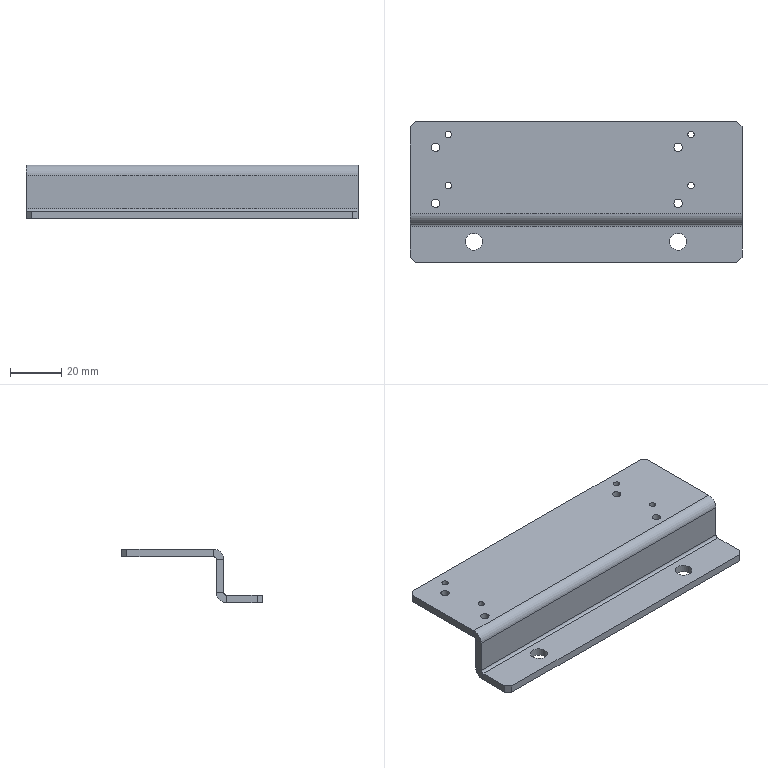Part | NX | 1 solid | 36 faces | box 130 x 55 x 21 mm | volume 27242 mm3 | plane 22 | cylinder 14 | commonest cylinder face diameters 2.5 x4 3.3 x4 2 x2 6.6 x2 8 x2
STEP:
#1=CARTESIAN_POINT('',(65.,-21.5,-4.));
#2=VERTEX_POINT('',#1);
#3=CARTESIAN_POINT('',(65.,-21.5,-17.));
#4=VERTEX_POINT('',#3);
#5=CARTESIAN_POINT('',(65.,-21.5,-18.));
#6=DIRECTION('',(0.,0.,-1.));
#7=VECTOR('',#6,1000.);
#8=LINE('',#5,#7);
#9=EDGE_CURVE('',#2,#4,#8,.T.);
#10=ORIENTED_EDGE('',*,*,#9,.T.);
#11=CARTESIAN_POINT('',(65.,-18.5,-17.));
#12=VERTEX_POINT('',#11);
#13=CARTESIAN_POINT('',(65.,-21.5,-17.));
#14=DIRECTION('',(0.,1.,0.));
#15=VECTOR('',#14,1000.);
#16=LINE('',#13,#15);
#17=EDGE_CURVE('',#4,#12,#16,.T.);
#18=ORIENTED_EDGE('',*,*,#17,.T.);
#19=CARTESIAN_POINT('',(65.,-18.5,-4.));
#20=VERTEX_POINT('',#19);
#21=CARTESIAN_POINT('',(65.,-18.5,-18.));
#22=DIRECTION('',(0.,0.,-1.));
#23=VECTOR('',#22,1000.);
#24=LINE('',#21,#23);
#25=EDGE_CURVE('',#20,#12,#24,.T.);
#26=ORIENTED_EDGE('',*,*,#25,.F.);
#27=CARTESIAN_POINT('',(65.,-18.5,-4.));
#28=DIRECTION('',(0.,-1.,0.));
#29=VECTOR('',#28,1000.);
#30=LINE('',#27,#29);
#31=EDGE_CURVE('',#20,#2,#30,.T.);
#32=ORIENTED_EDGE('',*,*,#31,.T.);
#33=EDGE_LOOP('',(#10,#18,#26,#32));
#34=FACE_BOUND('',#33,.T.);
#35=CARTESIAN_POINT('',(65.,-21.5,-18.));
#36=DIRECTION('',(1.,0.,0.));
#37=DIRECTION('',(0.,0.,-1.));
#38=AXIS2_PLACEMENT_3D('',#35,#36,#37);
#39=PLANE('',#38);
#40=ADVANCED_FACE('',(#34),#39,.T.);
#41=CARTESIAN_POINT('',(-65.,-21.5,-17.));
#42=VERTEX_POINT('',#41);
#43=CARTESIAN_POINT('',(-65.,-21.5,-4.));
#44=VERTEX_POINT('',#43);
#45=CARTESIAN_POINT('',(-65.,-21.5,-3.));
#46=DIRECTION('',(0.,0.,1.));
#47=VECTOR('',#46,1000.);
#48=LINE('',#45,#47);
#49=EDGE_CURVE('',#42,#44,#48,.T.);
#50=ORIENTED_EDGE('',*,*,#49,.F.);
#51=CARTESIAN_POINT('',(65.,-21.5,-17.));
#52=DIRECTION('',(1.,0.,0.));
#53=VECTOR('',#52,1000.);
#54=LINE('',#51,#53);
#55=EDGE_CURVE('',#4,#42,#54,.F.);
#56=ORIENTED_EDGE('',*,*,#55,.F.);
#57=ORIENTED_EDGE('',*,*,#9,.F.);
#58=CARTESIAN_POINT('',(0.,-21.5,-4.));
#59=DIRECTION('',(-1.,0.,0.));
#60=VECTOR('',#59,1000.);
#61=LINE('',#58,#60);
#62=EDGE_CURVE('',#2,#44,#61,.T.);
#63=ORIENTED_EDGE('',*,*,#62,.T.);
#64=EDGE_LOOP('',(#50,#56,#57,#63));
#65=FACE_BOUND('',#64,.T.);
#66=CARTESIAN_POINT('',(0.,-21.5,0.));
#67=DIRECTION('',(0.,-1.,0.));
#68=DIRECTION('',(0.,0.,-1.));
#69=AXIS2_PLACEMENT_3D('',#66,#67,#68);
#70=PLANE('',#69);
#71=ADVANCED_FACE('',(#65),#70,.T.);
#72=CARTESIAN_POINT('',(-65.,-18.5,-17.));
#73=VERTEX_POINT('',#72);
#74=CARTESIAN_POINT('',(65.,-18.5,-17.));
#75=DIRECTION('',(1.,0.,0.));
#76=VECTOR('',#75,1000.);
#77=LINE('',#74,#76);
#78=EDGE_CURVE('',#12,#73,#77,.F.);
#79=ORIENTED_EDGE('',*,*,#78,.T.);
#80=CARTESIAN_POINT('',(-65.,-18.5,-4.));
#81=VERTEX_POINT('',#80);
#82=CARTESIAN_POINT('',(-65.,-18.5,-3.));
#83=DIRECTION('',(0.,0.,1.));
#84=VECTOR('',#83,1000.);
#85=LINE('',#82,#84);
#86=EDGE_CURVE('',#73,#81,#85,.T.);
#87=ORIENTED_EDGE('',*,*,#86,.T.);
#88=CARTESIAN_POINT('',(65.,-18.5,-4.));
#89=DIRECTION('',(-1.,0.,0.));
#90=VECTOR('',#89,1000.);
#91=LINE('',#88,#90);
#92=EDGE_CURVE('',#20,#81,#91,.T.);
#93=ORIENTED_EDGE('',*,*,#92,.F.);
#94=ORIENTED_EDGE('',*,*,#25,.T.);
#95=EDGE_LOOP('',(#79,#87,#93,#94));
#96=FACE_BOUND('',#95,.T.);
#97=CARTESIAN_POINT('',(0.,-18.5,0.));
#98=DIRECTION('',(0.,-1.,0.));
#99=DIRECTION('',(0.,0.,-1.));
#100=AXIS2_PLACEMENT_3D('',#97,#98,#99);
#101=PLANE('',#100);
#102=ADVANCED_FACE('',(#96),#101,.F.);
#103=CARTESIAN_POINT('',(-65.,16.5,0.));
#104=VERTEX_POINT('',#103);
#105=CARTESIAN_POINT('',(-65.,-17.5,0.));
#106=VERTEX_POINT('',#105);
#107=CARTESIAN_POINT('',(-65.,-18.5,0.));
#108=DIRECTION('',(0.,-1.,0.));
#109=VECTOR('',#108,1000.);
#110=LINE('',#107,#109);
#111=EDGE_CURVE('',#104,#106,#110,.T.);
#112=ORIENTED_EDGE('',*,*,#111,.F.);
#113=CARTESIAN_POINT('',(-65.,16.5,-3.));
#114=VERTEX_POINT('',#113);
#115=CARTESIAN_POINT('',(-65.,16.5,-3.));
#116=DIRECTION('',(0.,0.,-1.));
#117=VECTOR('',#116,1000.);
#118=LINE('',#115,#117);
#119=EDGE_CURVE('',#104,#114,#118,.T.);
#120=ORIENTED_EDGE('',*,*,#119,.T.);
#121=CARTESIAN_POINT('',(-65.,-17.5,-3.));
#122=VERTEX_POINT('',#121);
#123=CARTESIAN_POINT('',(-65.,-18.5,-3.));
#124=DIRECTION('',(0.,-1.,0.));
#125=VECTOR('',#124,1000.);
#126=LINE('',#123,#125);
#127=EDGE_CURVE('',#114,#122,#126,.T.);
#128=ORIENTED_EDGE('',*,*,#127,.T.);
#129=CARTESIAN_POINT('',(-65.,-17.5,-3.));
#130=DIRECTION('',(0.,0.,1.));
#131=VECTOR('',#130,1000.);
#132=LINE('',#129,#131);
#133=EDGE_CURVE('',#122,#106,#132,.T.);
#134=ORIENTED_EDGE('',*,*,#133,.T.);
#135=EDGE_LOOP('',(#112,#120,#128,#134));
#136=FACE_BOUND('',#135,.T.);
#137=CARTESIAN_POINT('',(-65.,-18.5,-3.));
#138=DIRECTION('',(-1.,0.,0.));
#139=DIRECTION('',(0.,0.,1.));
#140=AXIS2_PLACEMENT_3D('',#137,#138,#139);
#141=PLANE('',#140);
#142=ADVANCED_FACE('',(#136),#141,.T.);
#143=CARTESIAN_POINT('',(-51.25,-6.5,-3.));
#144=VERTEX_POINT('',#143);
#145=CARTESIAN_POINT('',(-50.,-6.5,-3.));
#146=DIRECTION('',(0.,0.,-1.));
#147=DIRECTION('',(-1.,0.,0.));
#148=AXIS2_PLACEMENT_3D('',#145,#146,#147);
#149=CIRCLE('',#148,1.25);
#150=EDGE_CURVE('',#144,#144,#149,.T.);
#151=ORIENTED_EDGE('',*,*,#150,.F.);
#152=EDGE_LOOP('',(#151));
#153=FACE_BOUND('',#152,.T.);
#154=CARTESIAN_POINT('',(-51.25,13.5,-3.));
#155=VERTEX_POINT('',#154);
#156=CARTESIAN_POINT('',(-50.,13.5,-3.));
#157=DIRECTION('',(0.,0.,-1.));
#158=DIRECTION('',(-1.,0.,0.));
#159=AXIS2_PLACEMENT_3D('',#156,#157,#158);
#160=CIRCLE('',#159,1.25);
#161=EDGE_CURVE('',#155,#155,#160,.T.);
#162=ORIENTED_EDGE('',*,*,#161,.F.);
#163=EDGE_LOOP('',(#162));
#164=FACE_BOUND('',#163,.T.);
#165=CARTESIAN_POINT('',(43.75,-6.5,-3.));
#166=VERTEX_POINT('',#165);
#167=CARTESIAN_POINT('',(45.,-6.5,-3.));
#168=DIRECTION('',(0.,0.,-1.));
#169=DIRECTION('',(-1.,0.,0.));
#170=AXIS2_PLACEMENT_3D('',#167,#168,#169);
#171=CIRCLE('',#170,1.25);
#172=EDGE_CURVE('',#166,#166,#171,.T.);
#173=ORIENTED_EDGE('',*,*,#172,.F.);
#174=EDGE_LOOP('',(#173));
#175=FACE_BOUND('',#174,.T.);
#176=CARTESIAN_POINT('',(43.75,13.5,-3.));
#177=VERTEX_POINT('',#176);
#178=CARTESIAN_POINT('',(45.,13.5,-3.));
#179=DIRECTION('',(0.,0.,-1.));
#180=DIRECTION('',(-1.,0.,0.));
#181=AXIS2_PLACEMENT_3D('',#178,#179,#180);
#182=CIRCLE('',#181,1.25);
#183=EDGE_CURVE('',#177,#177,#182,.T.);
#184=ORIENTED_EDGE('',*,*,#183,.F.);
#185=EDGE_LOOP('',(#184));
#186=FACE_BOUND('',#185,.T.);
#187=CARTESIAN_POINT('',(-56.65,-13.5,-3.));
#188=VERTEX_POINT('',#187);
#189=CARTESIAN_POINT('',(-55.,-13.5,-3.));
#190=DIRECTION('',(0.,0.,-1.));
#191=DIRECTION('',(-1.,0.,0.));
#192=AXIS2_PLACEMENT_3D('',#189,#190,#191);
#193=CIRCLE('',#192,1.65);
#194=EDGE_CURVE('',#188,#188,#193,.T.);
#195=ORIENTED_EDGE('',*,*,#194,.F.);
#196=EDGE_LOOP('',(#195));
#197=FACE_BOUND('',#196,.T.);
#198=CARTESIAN_POINT('',(-56.65,8.5,-3.));
#199=VERTEX_POINT('',#198);
#200=CARTESIAN_POINT('',(-55.,8.5,-3.));
#201=DIRECTION('',(0.,0.,-1.));
#202=DIRECTION('',(-1.,0.,0.));
#203=AXIS2_PLACEMENT_3D('',#200,#201,#202);
#204=CIRCLE('',#203,1.65);
#205=EDGE_CURVE('',#199,#199,#204,.T.);
#206=ORIENTED_EDGE('',*,*,#205,.F.);
#207=EDGE_LOOP('',(#206));
#208=FACE_BOUND('',#207,.T.);
#209=CARTESIAN_POINT('',(38.35,-13.5,-3.));
#210=VERTEX_POINT('',#209);
#211=CARTESIAN_POINT('',(40.,-13.5,-3.));
#212=DIRECTION('',(0.,0.,-1.));
#213=DIRECTION('',(-1.,0.,0.));
#214=AXIS2_PLACEMENT_3D('',#211,#212,#213);
#215=CIRCLE('',#214,1.65);
#216=EDGE_CURVE('',#210,#210,#215,.T.);
#217=ORIENTED_EDGE('',*,*,#216,.F.);
#218=EDGE_LOOP('',(#217));
#219=FACE_BOUND('',#218,.T.);
#220=CARTESIAN_POINT('',(38.35,8.5,-3.));
#221=VERTEX_POINT('',#220);
#222=CARTESIAN_POINT('',(40.,8.5,-3.));
#223=DIRECTION('',(0.,0.,-1.));
#224=DIRECTION('',(-1.,0.,0.));
#225=AXIS2_PLACEMENT_3D('',#222,#223,#224);
#226=CIRCLE('',#225,1.65);
#227=EDGE_CURVE('',#221,#221,#226,.T.);
#228=ORIENTED_EDGE('',*,*,#227,.F.);
#229=EDGE_LOOP('',(#228));
#230=FACE_BOUND('',#229,.T.);
#231=ORIENTED_EDGE('',*,*,#127,.F.);
#232=CARTESIAN_POINT('',(-63.,18.5,-3.));
#233=VERTEX_POINT('',#232);
#234=CARTESIAN_POINT('',(-40.75,40.75,-3.));
#235=DIRECTION('',(-0.7071,-0.7071,0.));
#236=VECTOR('',#235,1000.);
#237=LINE('',#234,#236);
#238=EDGE_CURVE('',#114,#233,#237,.F.);
#239=ORIENTED_EDGE('',*,*,#238,.T.);
#240=CARTESIAN_POINT('',(63.,18.5,-3.));
#241=VERTEX_POINT('',#240);
#242=CARTESIAN_POINT('',(-65.,18.5,-3.));
#243=DIRECTION('',(-1.,0.,0.));
#244=VECTOR('',#243,1000.);
#245=LINE('',#242,#244);
#246=EDGE_CURVE('',#241,#233,#245,.T.);
#247=ORIENTED_EDGE('',*,*,#246,.F.);
#248=CARTESIAN_POINT('',(65.,16.5,-3.));
#249=VERTEX_POINT('',#248);
#250=CARTESIAN_POINT('',(40.75,40.75,-3.));
#251=DIRECTION('',(-0.7071,0.7071,0.));
#252=VECTOR('',#251,1000.);
#253=LINE('',#250,#252);
#254=EDGE_CURVE('',#241,#249,#253,.F.);
#255=ORIENTED_EDGE('',*,*,#254,.T.);
#256=CARTESIAN_POINT('',(65.,-17.5,-3.));
#257=VERTEX_POINT('',#256);
#258=CARTESIAN_POINT('',(65.,-18.5,-3.));
#259=DIRECTION('',(0.,1.,0.));
#260=VECTOR('',#259,1000.);
#261=LINE('',#258,#260);
#262=EDGE_CURVE('',#257,#249,#261,.T.);
#263=ORIENTED_EDGE('',*,*,#262,.F.);
#264=CARTESIAN_POINT('',(-65.,-17.5,-3.));
#265=DIRECTION('',(-1.,0.,0.));
#266=VECTOR('',#265,1000.);
#267=LINE('',#264,#266);
#268=EDGE_CURVE('',#122,#257,#267,.F.);
#269=ORIENTED_EDGE('',*,*,#268,.F.);
#270=EDGE_LOOP('',(#231,#239,#247,#255,#263,#269));
#271=FACE_BOUND('',#270,.T.);
#272=CARTESIAN_POINT('',(0.,0.,-3.));
#273=DIRECTION('',(0.,0.,-1.));
#274=DIRECTION('',(-1.,0.,0.));
#275=AXIS2_PLACEMENT_3D('',#272,#273,#274);
#276=PLANE('',#275);
#277=ADVANCED_FACE('',(#153,#164,#175,#186,#197,#208,#219,#230,#271),#276,.T.);
#278=CARTESIAN_POINT('',(-51.25,-6.5,0.));
#279=VERTEX_POINT('',#278);
#280=CARTESIAN_POINT('',(-50.,-6.5,0.));
#281=DIRECTION('',(0.,0.,-1.));
#282=DIRECTION('',(-1.,0.,0.));
#283=AXIS2_PLACEMENT_3D('',#280,#281,#282);
#284=CIRCLE('',#283,1.25);
#285=EDGE_CURVE('',#279,#279,#284,.T.);
#286=ORIENTED_EDGE('',*,*,#285,.T.);
#287=EDGE_LOOP('',(#286));
#288=FACE_BOUND('',#287,.T.);
#289=CARTESIAN_POINT('',(-51.25,13.5,0.));
#290=VERTEX_POINT('',#289);
#291=CARTESIAN_POINT('',(-50.,13.5,0.));
#292=DIRECTION('',(0.,0.,-1.));
#293=DIRECTION('',(-1.,0.,0.));
#294=AXIS2_PLACEMENT_3D('',#291,#292,#293);
#295=CIRCLE('',#294,1.25);
#296=EDGE_CURVE('',#290,#290,#295,.T.);
#297=ORIENTED_EDGE('',*,*,#296,.T.);
#298=EDGE_LOOP('',(#297));
#299=FACE_BOUND('',#298,.T.);
#300=CARTESIAN_POINT('',(43.75,-6.5,0.));
#301=VERTEX_POINT('',#300);
#302=CARTESIAN_POINT('',(45.,-6.5,0.));
#303=DIRECTION('',(0.,0.,-1.));
#304=DIRECTION('',(-1.,0.,0.));
#305=AXIS2_PLACEMENT_3D('',#302,#303,#304);
#306=CIRCLE('',#305,1.25);
#307=EDGE_CURVE('',#301,#301,#306,.T.);
#308=ORIENTED_EDGE('',*,*,#307,.T.);
#309=EDGE_LOOP('',(#308));
#310=FACE_BOUND('',#309,.T.);
#311=CARTESIAN_POINT('',(43.75,13.5,0.));
#312=VERTEX_POINT('',#311);
#313=CARTESIAN_POINT('',(45.,13.5,0.));
#314=DIRECTION('',(0.,0.,-1.));
#315=DIRECTION('',(-1.,0.,0.));
#316=AXIS2_PLACEMENT_3D('',#313,#314,#315);
#317=CIRCLE('',#316,1.25);
#318=EDGE_CURVE('',#312,#312,#317,.T.);
#319=ORIENTED_EDGE('',*,*,#318,.T.);
#320=EDGE_LOOP('',(#319));
#321=FACE_BOUND('',#320,.T.);
#322=CARTESIAN_POINT('',(-56.65,-13.5,0.));
#323=VERTEX_POINT('',#322);
#324=CARTESIAN_POINT('',(-55.,-13.5,0.));
#325=DIRECTION('',(0.,0.,-1.));
#326=DIRECTION('',(-1.,0.,0.));
#327=AXIS2_PLACEMENT_3D('',#324,#325,#326);
#328=CIRCLE('',#327,1.65);
#329=EDGE_CURVE('',#323,#323,#328,.T.);
#330=ORIENTED_EDGE('',*,*,#329,.T.);
#331=EDGE_LOOP('',(#330));
#332=FACE_BOUND('',#331,.T.);
#333=CARTESIAN_POINT('',(-56.65,8.5,0.));
#334=VERTEX_POINT('',#333);
#335=CARTESIAN_POINT('',(-55.,8.5,0.));
#336=DIRECTION('',(0.,0.,-1.));
#337=DIRECTION('',(-1.,0.,0.));
#338=AXIS2_PLACEMENT_3D('',#335,#336,#337);
#339=CIRCLE('',#338,1.65);
#340=EDGE_CURVE('',#334,#334,#339,.T.);
#341=ORIENTED_EDGE('',*,*,#340,.T.);
#342=EDGE_LOOP('',(#341));
#343=FACE_BOUND('',#342,.T.);
#344=CARTESIAN_POINT('',(38.35,-13.5,0.));
#345=VERTEX_POINT('',#344);
#346=CARTESIAN_POINT('',(40.,-13.5,0.));
#347=DIRECTION('',(0.,0.,-1.));
#348=DIRECTION('',(-1.,0.,0.));
#349=AXIS2_PLACEMENT_3D('',#346,#347,#348);
#350=CIRCLE('',#349,1.65);
#351=EDGE_CURVE('',#345,#345,#350,.T.);
#352=ORIENTED_EDGE('',*,*,#351,.T.);
#353=EDGE_LOOP('',(#352));
#354=FACE_BOUND('',#353,.T.);
#355=CARTESIAN_POINT('',(38.35,8.5,0.));
#356=VERTEX_POINT('',#355);
#357=CARTESIAN_POINT('',(40.,8.5,0.));
#358=DIRECTION('',(0.,0.,-1.));
#359=DIRECTION('',(-1.,0.,0.));
#360=AXIS2_PLACEMENT_3D('',#357,#358,#359);
#361=CIRCLE('',#360,1.65);
#362=EDGE_CURVE('',#356,#356,#361,.T.);
#363=ORIENTED_EDGE('',*,*,#362,.T.);
#364=EDGE_LOOP('',(#363));
#365=FACE_BOUND('',#364,.T.);
#366=CARTESIAN_POINT('',(63.,18.5,0.));
#367=VERTEX_POINT('',#366);
#368=CARTESIAN_POINT('',(-63.,18.5,0.));
#369=VERTEX_POINT('',#368);
#370=CARTESIAN_POINT('',(-65.,18.5,0.));
#371=DIRECTION('',(-1.,0.,0.));
#372=VECTOR('',#371,1000.);
#373=LINE('',#370,#372);
#374=EDGE_CURVE('',#367,#369,#373,.T.);
#375=ORIENTED_EDGE('',*,*,#374,.T.);
#376=CARTESIAN_POINT('',(-63.,18.5,0.));
#377=DIRECTION('',(0.7071,0.7071,0.));
#378=VECTOR('',#377,1000.);
#379=LINE('',#376,#378);
#380=EDGE_CURVE('',#369,#104,#379,.F.);
#381=ORIENTED_EDGE('',*,*,#380,.T.);
#382=ORIENTED_EDGE('',*,*,#111,.T.);
#383=CARTESIAN_POINT('',(65.,-17.5,0.));
#384=VERTEX_POINT('',#383);
#385=CARTESIAN_POINT('',(-65.,-17.5,0.));
#386=DIRECTION('',(-1.,0.,0.));
#387=VECTOR('',#386,1000.);
#388=LINE('',#385,#387);
#389=EDGE_CURVE('',#106,#384,#388,.F.);
#390=ORIENTED_EDGE('',*,*,#389,.T.);
#391=CARTESIAN_POINT('',(65.,16.5,0.));
#392=VERTEX_POINT('',#391);
#393=CARTESIAN_POINT('',(65.,-18.5,0.));
#394=DIRECTION('',(0.,1.,0.));
#395=VECTOR('',#394,1000.);
#396=LINE('',#393,#395);
#397=EDGE_CURVE('',#384,#392,#396,.T.);
#398=ORIENTED_EDGE('',*,*,#397,.T.);
#399=CARTESIAN_POINT('',(65.,16.5,0.));
#400=DIRECTION('',(0.7071,-0.7071,0.));
#401=VECTOR('',#400,1000.);
#402=LINE('',#399,#401);
#403=EDGE_CURVE('',#392,#367,#402,.F.);
#404=ORIENTED_EDGE('',*,*,#403,.T.);
#405=EDGE_LOOP('',(#375,#381,#382,#390,#398,#404));
#406=FACE_BOUND('',#405,.T.);
#407=CARTESIAN_POINT('',(0.,0.,0.));
#408=DIRECTION('',(0.,0.,-1.));
#409=DIRECTION('',(-1.,0.,0.));
#410=AXIS2_PLACEMENT_3D('',#407,#408,#409);
#411=PLANE('',#410);
#412=ADVANCED_FACE('',(#288,#299,#310,#321,#332,#343,#354,#365,#406),#411,.F.);
#413=ORIENTED_EDGE('',*,*,#262,.T.);
#414=CARTESIAN_POINT('',(65.,16.5,-3.));
#415=DIRECTION('',(0.,0.,1.));
#416=VECTOR('',#415,1000.);
#417=LINE('',#414,#416);
#418=EDGE_CURVE('',#249,#392,#417,.T.);
#419=ORIENTED_EDGE('',*,*,#418,.T.);
#420=ORIENTED_EDGE('',*,*,#397,.F.);
#421=CARTESIAN_POINT('',(65.,-17.5,-3.));
#422=DIRECTION('',(0.,0.,1.));
#423=VECTOR('',#422,1000.);
#424=LINE('',#421,#423);
#425=EDGE_CURVE('',#257,#384,#424,.T.);
#426=ORIENTED_EDGE('',*,*,#425,.F.);
#427=EDGE_LOOP('',(#413,#419,#420,#426));
#428=FACE_BOUND('',#427,.T.);
#429=CARTESIAN_POINT('',(65.,-18.5,-3.));
#430=DIRECTION('',(1.,0.,0.));
#431=DIRECTION('',(0.,0.,-1.));
#432=AXIS2_PLACEMENT_3D('',#429,#430,#431);
#433=PLANE('',#432);
#434=ADVANCED_FACE('',(#428),#433,.T.);
#435=ORIENTED_EDGE('',*,*,#246,.T.);
#436=CARTESIAN_POINT('',(-63.,18.5,-3.));
#437=DIRECTION('',(0.,0.,1.));
#438=VECTOR('',#437,1000.);
#439=LINE('',#436,#438);
#440=EDGE_CURVE('',#233,#369,#439,.T.);
#441=ORIENTED_EDGE('',*,*,#440,.T.);
#442=ORIENTED_EDGE('',*,*,#374,.F.);
#443=CARTESIAN_POINT('',(63.,18.5,-3.));
#444=DIRECTION('',(0.,0.,-1.));
#445=VECTOR('',#444,1000.);
#446=LINE('',#443,#445);
#447=EDGE_CURVE('',#367,#241,#446,.T.);
#448=ORIENTED_EDGE('',*,*,#447,.T.);
#449=EDGE_LOOP('',(#435,#441,#442,#448));
#450=FACE_BOUND('',#449,.T.);
#451=CARTESIAN_POINT('',(-65.,18.5,-3.));
#452=DIRECTION('',(0.,1.,0.));
#453=DIRECTION('',(0.,0.,1.));
#454=AXIS2_PLACEMENT_3D('',#451,#452,#453);
#455=PLANE('',#454);
#456=ADVANCED_FACE('',(#450),#455,.T.);
#457=ORIENTED_EDGE('',*,*,#329,.F.);
#458=EDGE_LOOP('',(#457));
#459=FACE_BOUND('',#458,.T.);
#460=ORIENTED_EDGE('',*,*,#194,.T.);
#461=EDGE_LOOP('',(#460));
#462=FACE_BOUND('',#461,.T.);
#463=CARTESIAN_POINT('',(-55.,-13.5,-3.));
#464=DIRECTION('',(0.,0.,-1.));
#465=DIRECTION('',(-1.,0.,0.));
#466=AXIS2_PLACEMENT_3D('',#463,#464,#465);
#467=CYLINDRICAL_SURFACE('',#466,1.65);
#468=ADVANCED_FACE('',(#459,#462),#467,.F.);
#469=ORIENTED_EDGE('',*,*,#340,.F.);
#470=EDGE_LOOP('',(#469));
#471=FACE_BOUND('',#470,.T.);
#472=ORIENTED_EDGE('',*,*,#205,.T.);
#473=EDGE_LOOP('',(#472));
#474=FACE_BOUND('',#473,.T.);
#475=CARTESIAN_POINT('',(-55.,8.5,-3.));
#476=DIRECTION('',(0.,0.,-1.));
#477=DIRECTION('',(-1.,0.,0.));
#478=AXIS2_PLACEMENT_3D('',#475,#476,#477);
#479=CYLINDRICAL_SURFACE('',#478,1.65);
#480=ADVANCED_FACE('',(#471,#474),#479,.F.);
#481=ORIENTED_EDGE('',*,*,#351,.F.);
#482=EDGE_LOOP('',(#481));
#483=FACE_BOUND('',#482,.T.);
#484=ORIENTED_EDGE('',*,*,#216,.T.);
#485=EDGE_LOOP('',(#484));
#486=FACE_BOUND('',#485,.T.);
#487=CARTESIAN_POINT('',(40.,-13.5,-3.));
#488=DIRECTION('',(0.,0.,-1.));
#489=DIRECTION('',(-1.,0.,0.));
#490=AXIS2_PLACEMENT_3D('',#487,#488,#489);
#491=CYLINDRICAL_SURFACE('',#490,1.65);
#492=ADVANCED_FACE('',(#483,#486),#491,.F.);
#493=ORIENTED_EDGE('',*,*,#362,.F.);
#494=EDGE_LOOP('',(#493));
#495=FACE_BOUND('',#494,.T.);
#496=ORIENTED_EDGE('',*,*,#227,.T.);
#497=EDGE_LOOP('',(#496));
#498=FACE_BOUND('',#497,.T.);
#499=CARTESIAN_POINT('',(40.,8.5,-3.));
#500=DIRECTION('',(0.,0.,-1.));
#501=DIRECTION('',(-1.,0.,0.));
#502=AXIS2_PLACEMENT_3D('',#499,#500,#501);
#503=CYLINDRICAL_SURFACE('',#502,1.65);
#504=ADVANCED_FACE('',(#495,#498),#503,.F.);
#505=ORIENTED_EDGE('',*,*,#31,.F.);
#506=CARTESIAN_POINT('',(65.,-17.5,-4.));
#507=DIRECTION('',(-1.,0.,0.));
#508=DIRECTION('',(0.,0.,1.));
#509=AXIS2_PLACEMENT_3D('',#506,#507,#508);
#510=CIRCLE('',#509,1.);
#511=EDGE_CURVE('',#257,#20,#510,.F.);
#512=ORIENTED_EDGE('',*,*,#511,.F.);
#513=ORIENTED_EDGE('',*,*,#425,.T.);
#514=CARTESIAN_POINT('',(65.,-17.5,-4.));
#515=DIRECTION('',(-1.,0.,0.));
#516=DIRECTION('',(0.,0.,1.));
#517=AXIS2_PLACEMENT_3D('',#514,#515,#516);
#518=CIRCLE('',#517,4.);
#519=EDGE_CURVE('',#384,#2,#518,.F.);
#520=ORIENTED_EDGE('',*,*,#519,.T.);
#521=EDGE_LOOP('',(#505,#512,#513,#520));
#522=FACE_BOUND('',#521,.T.);
#523=CARTESIAN_POINT('',(65.,-17.5,-4.));
#524=DIRECTION('',(1.,0.,0.));
#525=DIRECTION('',(0.,0.,-1.));
#526=AXIS2_PLACEMENT_3D('',#523,#524,#525);
#527=PLANE('',#526);
#528=ADVANCED_FACE('',(#522),#527,.T.);
#529=CARTESIAN_POINT('',(-65.,-17.5,-4.));
#530=DIRECTION('',(-1.,0.,0.));
#531=DIRECTION('',(0.,0.,1.));
#532=AXIS2_PLACEMENT_3D('',#529,#530,#531);
#533=CIRCLE('',#532,1.);
#534=EDGE_CURVE('',#81,#122,#533,.T.);
#535=ORIENTED_EDGE('',*,*,#534,.F.);
#536=CARTESIAN_POINT('',(-65.,-18.5,-4.));
#537=DIRECTION('',(0.,-1.,0.));
#538=VECTOR('',#537,1000.);
#539=LINE('',#536,#538);
#540=EDGE_CURVE('',#81,#44,#539,.T.);
#541=ORIENTED_EDGE('',*,*,#540,.T.);
#542=CARTESIAN_POINT('',(-65.,-17.5,-4.));
#543=DIRECTION('',(-1.,0.,0.));
#544=DIRECTION('',(0.,0.,1.));
#545=AXIS2_PLACEMENT_3D('',#542,#543,#544);
#546=CIRCLE('',#545,4.);
#547=EDGE_CURVE('',#44,#106,#546,.T.);
#548=ORIENTED_EDGE('',*,*,#547,.T.);
#549=ORIENTED_EDGE('',*,*,#133,.F.);
#550=EDGE_LOOP('',(#535,#541,#548,#549));
#551=FACE_BOUND('',#550,.T.);
#552=CARTESIAN_POINT('',(-65.,-17.5,-4.));
#553=DIRECTION('',(1.,0.,0.));
#554=DIRECTION('',(0.,0.,-1.));
#555=AXIS2_PLACEMENT_3D('',#552,#553,#554);
#556=PLANE('',#555);
#557=ADVANCED_FACE('',(#551),#556,.F.);
#558=ORIENTED_EDGE('',*,*,#389,.F.);
#559=ORIENTED_EDGE('',*,*,#547,.F.);
#560=ORIENTED_EDGE('',*,*,#62,.F.);
#561=ORIENTED_EDGE('',*,*,#519,.F.);
#562=EDGE_LOOP('',(#558,#559,#560,#561));
#563=FACE_BOUND('',#562,.T.);
#564=CARTESIAN_POINT('',(-65.,-17.5,-4.));
#565=DIRECTION('',(-1.,0.,0.));
#566=DIRECTION('',(0.,-1.,0.));
#567=AXIS2_PLACEMENT_3D('',#564,#565,#566);
#568=CYLINDRICAL_SURFACE('',#567,4.);
#569=ADVANCED_FACE('',(#563),#568,.T.);
#570=ORIENTED_EDGE('',*,*,#268,.T.);
#571=ORIENTED_EDGE('',*,*,#511,.T.);
#572=ORIENTED_EDGE('',*,*,#92,.T.);
#573=ORIENTED_EDGE('',*,*,#534,.T.);
#574=EDGE_LOOP('',(#570,#571,#572,#573));
#575=FACE_BOUND('',#574,.T.);
#576=CARTESIAN_POINT('',(-65.,-17.5,-4.));
#577=DIRECTION('',(-1.,0.,0.));
#578=DIRECTION('',(0.,-1.,0.));
#579=AXIS2_PLACEMENT_3D('',#576,#577,#578);
#580=CYLINDRICAL_SURFACE('',#579,1.);
#581=ADVANCED_FACE('',(#575),#580,.F.);
#582=CARTESIAN_POINT('',(-65.,-21.5,-17.));
#583=DIRECTION('',(0.,1.,0.));
#584=VECTOR('',#583,1000.);
#585=LINE('',#582,#584);
#586=EDGE_CURVE('',#42,#73,#585,.T.);
#587=ORIENTED_EDGE('',*,*,#586,.F.);
#588=ORIENTED_EDGE('',*,*,#49,.T.);
#589=ORIENTED_EDGE('',*,*,#540,.F.);
#590=ORIENTED_EDGE('',*,*,#86,.F.);
#591=EDGE_LOOP('',(#587,#588,#589,#590));
#592=FACE_BOUND('',#591,.T.);
#593=CARTESIAN_POINT('',(-65.,-21.5,-3.));
#594=DIRECTION('',(-1.,0.,0.));
#595=DIRECTION('',(0.,0.,1.));
#596=AXIS2_PLACEMENT_3D('',#593,#594,#595);
#597=PLANE('',#596);
#598=ADVANCED_FACE('',(#592),#597,.T.);
#599=CARTESIAN_POINT('',(-65.,-22.5,-18.));
#600=VERTEX_POINT('',#599);
#601=CARTESIAN_POINT('',(-65.,-22.5,-21.));
#602=VERTEX_POINT('',#601);
#603=CARTESIAN_POINT('',(-65.,-22.5,-18.));
#604=DIRECTION('',(0.,0.,-1.));
#605=VECTOR('',#604,1000.);
#606=LINE('',#603,#605);
#607=EDGE_CURVE('',#600,#602,#606,.T.);
#608=ORIENTED_EDGE('',*,*,#607,.F.);
#609=CARTESIAN_POINT('',(-65.,-22.5,-17.));
#610=DIRECTION('',(1.,0.,0.));
#611=DIRECTION('',(0.,0.,-1.));
#612=AXIS2_PLACEMENT_3D('',#609,#610,#611);
#613=CIRCLE('',#612,1.);
#614=EDGE_CURVE('',#42,#600,#613,.F.);
#615=ORIENTED_EDGE('',*,*,#614,.F.);
#616=ORIENTED_EDGE('',*,*,#586,.T.);
#617=CARTESIAN_POINT('',(-65.,-22.5,-17.));
#618=DIRECTION('',(1.,0.,0.));
#619=DIRECTION('',(0.,0.,-1.));
#620=AXIS2_PLACEMENT_3D('',#617,#618,#619);
#621=CIRCLE('',#620,4.);
#622=EDGE_CURVE('',#73,#602,#621,.F.);
#623=ORIENTED_EDGE('',*,*,#622,.T.);
#624=EDGE_LOOP('',(#608,#615,#616,#623));
#625=FACE_BOUND('',#624,.T.);
#626=CARTESIAN_POINT('',(-65.,-22.5,-17.));
#627=DIRECTION('',(-1.,0.,0.));
#628=DIRECTION('',(0.,0.,1.));
#629=AXIS2_PLACEMENT_3D('',#626,#627,#628);
#630=PLANE('',#629);
#631=ADVANCED_FACE('',(#625),#630,.T.);
#632=CARTESIAN_POINT('',(65.,-22.5,-18.));
#633=VERTEX_POINT('',#632);
#634=CARTESIAN_POINT('',(65.,-22.5,-17.));
#635=DIRECTION('',(1.,0.,0.));
#636=DIRECTION('',(0.,0.,-1.));
#637=AXIS2_PLACEMENT_3D('',#634,#635,#636);
#638=CIRCLE('',#637,1.);
#639=EDGE_CURVE('',#633,#4,#638,.T.);
#640=ORIENTED_EDGE('',*,*,#639,.F.);
#641=CARTESIAN_POINT('',(65.,-22.5,-21.));
#642=VERTEX_POINT('',#641);
#643=CARTESIAN_POINT('',(65.,-22.5,-18.));
#644=DIRECTION('',(0.,0.,-1.));
#645=VECTOR('',#644,1000.);
#646=LINE('',#643,#645);
#647=EDGE_CURVE('',#633,#642,#646,.T.);
#648=ORIENTED_EDGE('',*,*,#647,.T.);
#649=CARTESIAN_POINT('',(65.,-22.5,-17.));
#650=DIRECTION('',(1.,0.,0.));
#651=DIRECTION('',(0.,0.,-1.));
#652=AXIS2_PLACEMENT_3D('',#649,#650,#651);
#653=CIRCLE('',#652,4.);
#654=EDGE_CURVE('',#642,#12,#653,.T.);
#655=ORIENTED_EDGE('',*,*,#654,.T.);
#656=ORIENTED_EDGE('',*,*,#17,.F.);
#657=EDGE_LOOP('',(#640,#648,#655,#656));
#658=FACE_BOUND('',#657,.T.);
#659=CARTESIAN_POINT('',(65.,-22.5,-17.));
#660=DIRECTION('',(-1.,0.,0.));
#661=DIRECTION('',(0.,0.,1.));
#662=AXIS2_PLACEMENT_3D('',#659,#660,#661);
#663=PLANE('',#662);
#664=ADVANCED_FACE('',(#658),#663,.F.);
#665=ORIENTED_EDGE('',*,*,#78,.F.);
#666=ORIENTED_EDGE('',*,*,#654,.F.);
#667=CARTESIAN_POINT('',(0.,-22.5,-21.));
#668=DIRECTION('',(1.,0.,0.));
#669=VECTOR('',#668,1000.);
#670=LINE('',#667,#669);
#671=EDGE_CURVE('',#602,#642,#670,.T.);
#672=ORIENTED_EDGE('',*,*,#671,.F.);
#673=ORIENTED_EDGE('',*,*,#622,.F.);
#674=EDGE_LOOP('',(#665,#666,#672,#673));
#675=FACE_BOUND('',#674,.T.);
#676=CARTESIAN_POINT('',(65.,-22.5,-17.));
#677=DIRECTION('',(1.,0.,0.));
#678=DIRECTION('',(0.,0.,-1.));
#679=AXIS2_PLACEMENT_3D('',#676,#677,#678);
#680=CYLINDRICAL_SURFACE('',#679,4.);
#681=ADVANCED_FACE('',(#675),#680,.T.);
#682=ORIENTED_EDGE('',*,*,#55,.T.);
#683=ORIENTED_EDGE('',*,*,#614,.T.);
#684=CARTESIAN_POINT('',(-65.,-22.5,-18.));
#685=DIRECTION('',(1.,0.,0.));
#686=VECTOR('',#685,1000.);
#687=LINE('',#684,#686);
#688=EDGE_CURVE('',#600,#633,#687,.T.);
#689=ORIENTED_EDGE('',*,*,#688,.T.);
#690=ORIENTED_EDGE('',*,*,#639,.T.);
#691=EDGE_LOOP('',(#682,#683,#689,#690));
#692=FACE_BOUND('',#691,.T.);
#693=CARTESIAN_POINT('',(65.,-22.5,-17.));
#694=DIRECTION('',(1.,0.,0.));
#695=DIRECTION('',(0.,0.,-1.));
#696=AXIS2_PLACEMENT_3D('',#693,#694,#695);
#697=CYLINDRICAL_SURFACE('',#696,1.);
#698=ADVANCED_FACE('',(#692),#697,.F.);
#699=CARTESIAN_POINT('',(65.,-34.5,-18.));
#700=VERTEX_POINT('',#699);
#701=CARTESIAN_POINT('',(65.,-21.5,-18.));
#702=DIRECTION('',(0.,1.,0.));
#703=VECTOR('',#702,1000.);
#704=LINE('',#701,#703);
#705=EDGE_CURVE('',#700,#633,#704,.T.);
#706=ORIENTED_EDGE('',*,*,#705,.F.);
#707=CARTESIAN_POINT('',(65.,-34.5,-21.));
#708=VERTEX_POINT('',#707);
#709=CARTESIAN_POINT('',(65.,-34.5,-21.));
#710=DIRECTION('',(0.,0.,-1.));
#711=VECTOR('',#710,1000.);
#712=LINE('',#709,#711);
#713=EDGE_CURVE('',#700,#708,#712,.T.);
#714=ORIENTED_EDGE('',*,*,#713,.T.);
#715=CARTESIAN_POINT('',(65.,-21.5,-21.));
#716=DIRECTION('',(0.,1.,0.));
#717=VECTOR('',#716,1000.);
#718=LINE('',#715,#717);
#719=EDGE_CURVE('',#708,#642,#718,.T.);
#720=ORIENTED_EDGE('',*,*,#719,.T.);
#721=ORIENTED_EDGE('',*,*,#647,.F.);
#722=EDGE_LOOP('',(#706,#714,#720,#721));
#723=FACE_BOUND('',#722,.T.);
#724=CARTESIAN_POINT('',(65.,-21.5,-21.));
#725=DIRECTION('',(1.,0.,0.));
#726=DIRECTION('',(0.,0.,-1.));
#727=AXIS2_PLACEMENT_3D('',#724,#725,#726);
#728=PLANE('',#727);
#729=ADVANCED_FACE('',(#723),#728,.T.);
#730=CARTESIAN_POINT('',(-65.,-34.5,-21.));
#731=VERTEX_POINT('',#730);
#732=CARTESIAN_POINT('',(-65.,-36.5,-21.));
#733=DIRECTION('',(0.,-1.,0.));
#734=VECTOR('',#733,1000.);
#735=LINE('',#732,#734);
#736=EDGE_CURVE('',#602,#731,#735,.T.);
#737=ORIENTED_EDGE('',*,*,#736,.T.);
#738=CARTESIAN_POINT('',(-65.,-34.5,-18.));
#739=VERTEX_POINT('',#738);
#740=CARTESIAN_POINT('',(-65.,-34.5,-21.));
#741=DIRECTION('',(0.,0.,1.));
#742=VECTOR('',#741,1000.);
#743=LINE('',#740,#742);
#744=EDGE_CURVE('',#731,#739,#743,.T.);
#745=ORIENTED_EDGE('',*,*,#744,.T.);
#746=CARTESIAN_POINT('',(-65.,-36.5,-18.));
#747=DIRECTION('',(0.,-1.,0.));
#748=VECTOR('',#747,1000.);
#749=LINE('',#746,#748);
#750=EDGE_CURVE('',#600,#739,#749,.T.);
#751=ORIENTED_EDGE('',*,*,#750,.F.);
#752=ORIENTED_EDGE('',*,*,#607,.T.);
#753=EDGE_LOOP('',(#737,#745,#751,#752));
#754=FACE_BOUND('',#753,.T.);
#755=CARTESIAN_POINT('',(-65.,-36.5,-21.));
#756=DIRECTION('',(-1.,0.,0.));
#757=DIRECTION('',(0.,0.,1.));
#758=AXIS2_PLACEMENT_3D('',#755,#756,#757);
#759=PLANE('',#758);
#760=ADVANCED_FACE('',(#754),#759,.T.);
#761=CARTESIAN_POINT('',(-43.3,-28.5,-21.));
#762=VERTEX_POINT('',#761);
#763=CARTESIAN_POINT('',(-40.,-28.5,-21.));
#764=DIRECTION('',(0.,0.,-1.));
#765=DIRECTION('',(-1.,0.,0.));
#766=AXIS2_PLACEMENT_3D('',#763,#764,#765);
#767=CIRCLE('',#766,3.3);
#768=EDGE_CURVE('',#762,#762,#767,.T.);
#769=ORIENTED_EDGE('',*,*,#768,.F.);
#770=EDGE_LOOP('',(#769));
#771=FACE_BOUND('',#770,.T.);
#772=CARTESIAN_POINT('',(36.7,-28.5,-21.));
#773=VERTEX_POINT('',#772);
#774=CARTESIAN_POINT('',(40.,-28.5,-21.));
#775=DIRECTION('',(0.,0.,-1.));
#776=DIRECTION('',(-1.,0.,0.));
#777=AXIS2_PLACEMENT_3D('',#774,#775,#776);
#778=CIRCLE('',#777,3.3);
#779=EDGE_CURVE('',#773,#773,#778,.T.);
#780=ORIENTED_EDGE('',*,*,#779,.F.);
#781=EDGE_LOOP('',(#780));
#782=FACE_BOUND('',#781,.T.);
#783=ORIENTED_EDGE('',*,*,#719,.F.);
#784=CARTESIAN_POINT('',(63.,-36.5,-21.));
#785=VERTEX_POINT('',#784);
#786=CARTESIAN_POINT('',(49.75,-49.75,-21.));
#787=DIRECTION('',(0.7071,0.7071,0.));
#788=VECTOR('',#787,1000.);
#789=LINE('',#786,#788);
#790=EDGE_CURVE('',#708,#785,#789,.F.);
#791=ORIENTED_EDGE('',*,*,#790,.T.);
#792=CARTESIAN_POINT('',(-63.,-36.5,-21.));
#793=VERTEX_POINT('',#792);
#794=CARTESIAN_POINT('',(65.,-36.5,-21.));
#795=DIRECTION('',(1.,0.,0.));
#796=VECTOR('',#795,1000.);
#797=LINE('',#794,#796);
#798=EDGE_CURVE('',#793,#785,#797,.T.);
#799=ORIENTED_EDGE('',*,*,#798,.F.);
#800=CARTESIAN_POINT('',(-49.75,-49.75,-21.));
#801=DIRECTION('',(0.7071,-0.7071,0.));
#802=VECTOR('',#801,1000.);
#803=LINE('',#800,#802);
#804=EDGE_CURVE('',#793,#731,#803,.F.);
#805=ORIENTED_EDGE('',*,*,#804,.T.);
#806=ORIENTED_EDGE('',*,*,#736,.F.);
#807=ORIENTED_EDGE('',*,*,#671,.T.);
#808=EDGE_LOOP('',(#783,#791,#799,#805,#806,#807));
#809=FACE_BOUND('',#808,.T.);
#810=CARTESIAN_POINT('',(0.,0.,-21.));
#811=DIRECTION('',(0.,0.,-1.));
#812=DIRECTION('',(-1.,0.,0.));
#813=AXIS2_PLACEMENT_3D('',#810,#811,#812);
#814=PLANE('',#813);
#815=ADVANCED_FACE('',(#771,#782,#809),#814,.T.);
#816=CARTESIAN_POINT('',(-36.7,-28.5,-18.));
#817=VERTEX_POINT('',#816);
#818=CARTESIAN_POINT('',(-40.,-28.5,-18.));
#819=DIRECTION('',(0.,0.,1.));
#820=DIRECTION('',(1.,0.,0.));
#821=AXIS2_PLACEMENT_3D('',#818,#819,#820);
#822=CIRCLE('',#821,3.3);
#823=EDGE_CURVE('',#817,#817,#822,.T.);
#824=ORIENTED_EDGE('',*,*,#823,.F.);
#825=EDGE_LOOP('',(#824));
#826=FACE_BOUND('',#825,.T.);
#827=CARTESIAN_POINT('',(43.3,-28.5,-18.));
#828=VERTEX_POINT('',#827);
#829=CARTESIAN_POINT('',(40.,-28.5,-18.));
#830=DIRECTION('',(0.,0.,1.));
#831=DIRECTION('',(1.,0.,0.));
#832=AXIS2_PLACEMENT_3D('',#829,#830,#831);
#833=CIRCLE('',#832,3.3);
#834=EDGE_CURVE('',#828,#828,#833,.T.);
#835=ORIENTED_EDGE('',*,*,#834,.F.);
#836=EDGE_LOOP('',(#835));
#837=FACE_BOUND('',#836,.T.);
#838=CARTESIAN_POINT('',(-63.,-36.5,-18.));
#839=VERTEX_POINT('',#838);
#840=CARTESIAN_POINT('',(63.,-36.5,-18.));
#841=VERTEX_POINT('',#840);
#842=CARTESIAN_POINT('',(65.,-36.5,-18.));
#843=DIRECTION('',(1.,0.,0.));
#844=VECTOR('',#843,1000.);
#845=LINE('',#842,#844);
#846=EDGE_CURVE('',#839,#841,#845,.T.);
#847=ORIENTED_EDGE('',*,*,#846,.T.);
#848=CARTESIAN_POINT('',(63.,-36.5,-18.));
#849=DIRECTION('',(-0.7071,-0.7071,0.));
#850=VECTOR('',#849,1000.);
#851=LINE('',#848,#850);
#852=EDGE_CURVE('',#841,#700,#851,.F.);
#853=ORIENTED_EDGE('',*,*,#852,.T.);
#854=ORIENTED_EDGE('',*,*,#705,.T.);
#855=ORIENTED_EDGE('',*,*,#688,.F.);
#856=ORIENTED_EDGE('',*,*,#750,.T.);
#857=CARTESIAN_POINT('',(-65.,-34.5,-18.));
#858=DIRECTION('',(-0.7071,0.7071,0.));
#859=VECTOR('',#858,1000.);
#860=LINE('',#857,#859);
#861=EDGE_CURVE('',#739,#839,#860,.F.);
#862=ORIENTED_EDGE('',*,*,#861,.T.);
#863=EDGE_LOOP('',(#847,#853,#854,#855,#856,#862));
#864=FACE_BOUND('',#863,.T.);
#865=CARTESIAN_POINT('',(0.,0.,-18.));
#866=DIRECTION('',(0.,0.,-1.));
#867=DIRECTION('',(-1.,0.,0.));
#868=AXIS2_PLACEMENT_3D('',#865,#866,#867);
#869=PLANE('',#868);
#870=ADVANCED_FACE('',(#826,#837,#864),#869,.F.);
#871=ORIENTED_EDGE('',*,*,#798,.T.);
#872=CARTESIAN_POINT('',(63.,-36.5,-21.));
#873=DIRECTION('',(0.,0.,1.));
#874=VECTOR('',#873,1000.);
#875=LINE('',#872,#874);
#876=EDGE_CURVE('',#785,#841,#875,.T.);
#877=ORIENTED_EDGE('',*,*,#876,.T.);
#878=ORIENTED_EDGE('',*,*,#846,.F.);
#879=CARTESIAN_POINT('',(-63.,-36.5,-21.));
#880=DIRECTION('',(0.,0.,-1.));
#881=VECTOR('',#880,1000.);
#882=LINE('',#879,#881);
#883=EDGE_CURVE('',#839,#793,#882,.T.);
#884=ORIENTED_EDGE('',*,*,#883,.T.);
#885=EDGE_LOOP('',(#871,#877,#878,#884));
#886=FACE_BOUND('',#885,.T.);
#887=CARTESIAN_POINT('',(65.,-36.5,-21.));
#888=DIRECTION('',(0.,-1.,0.));
#889=DIRECTION('',(0.,0.,-1.));
#890=AXIS2_PLACEMENT_3D('',#887,#888,#889);
#891=PLANE('',#890);
#892=ADVANCED_FACE('',(#886),#891,.T.);
#893=ORIENTED_EDGE('',*,*,#779,.T.);
#894=EDGE_LOOP('',(#893));
#895=FACE_BOUND('',#894,.T.);
#896=ORIENTED_EDGE('',*,*,#834,.T.);
#897=EDGE_LOOP('',(#896));
#898=FACE_BOUND('',#897,.T.);
#899=CARTESIAN_POINT('',(40.,-28.5,-18.));
#900=DIRECTION('',(0.,0.,1.));
#901=DIRECTION('',(1.,0.,0.));
#902=AXIS2_PLACEMENT_3D('',#899,#900,#901);
#903=CYLINDRICAL_SURFACE('',#902,3.3);
#904=ADVANCED_FACE('',(#895,#898),#903,.F.);
#905=ORIENTED_EDGE('',*,*,#768,.T.);
#906=EDGE_LOOP('',(#905));
#907=FACE_BOUND('',#906,.T.);
#908=ORIENTED_EDGE('',*,*,#823,.T.);
#909=EDGE_LOOP('',(#908));
#910=FACE_BOUND('',#909,.T.);
#911=CARTESIAN_POINT('',(-40.,-28.5,-18.));
#912=DIRECTION('',(0.,0.,1.));
#913=DIRECTION('',(1.,0.,0.));
#914=AXIS2_PLACEMENT_3D('',#911,#912,#913);
#915=CYLINDRICAL_SURFACE('',#914,3.3);
#916=ADVANCED_FACE('',(#907,#910),#915,.F.);
#917=ORIENTED_EDGE('',*,*,#790,.F.);
#918=ORIENTED_EDGE('',*,*,#713,.F.);
#919=ORIENTED_EDGE('',*,*,#852,.F.);
#920=ORIENTED_EDGE('',*,*,#876,.F.);
#921=EDGE_LOOP('',(#917,#918,#919,#920));
#922=FACE_BOUND('',#921,.T.);
#923=CARTESIAN_POINT('',(63.,-36.5,-21.));
#924=DIRECTION('',(-0.7071,0.7071,0.));
#925=DIRECTION('',(0.,0.,1.));
#926=AXIS2_PLACEMENT_3D('',#923,#924,#925);
#927=PLANE('',#926);
#928=ADVANCED_FACE('',(#922),#927,.F.);
#929=ORIENTED_EDGE('',*,*,#804,.F.);
#930=ORIENTED_EDGE('',*,*,#883,.F.);
#931=ORIENTED_EDGE('',*,*,#861,.F.);
#932=ORIENTED_EDGE('',*,*,#744,.F.);
#933=EDGE_LOOP('',(#929,#930,#931,#932));
#934=FACE_BOUND('',#933,.T.);
#935=CARTESIAN_POINT('',(-65.,-34.5,-21.));
#936=DIRECTION('',(0.7071,0.7071,0.));
#937=DIRECTION('',(0.,0.,1.));
#938=AXIS2_PLACEMENT_3D('',#935,#936,#937);
#939=PLANE('',#938);
#940=ADVANCED_FACE('',(#934),#939,.F.);
#941=ORIENTED_EDGE('',*,*,#238,.F.);
#942=ORIENTED_EDGE('',*,*,#119,.F.);
#943=ORIENTED_EDGE('',*,*,#380,.F.);
#944=ORIENTED_EDGE('',*,*,#440,.F.);
#945=EDGE_LOOP('',(#941,#942,#943,#944));
#946=FACE_BOUND('',#945,.T.);
#947=CARTESIAN_POINT('',(-63.,18.5,-3.));
#948=DIRECTION('',(0.7071,-0.7071,0.));
#949=DIRECTION('',(0.,0.,1.));
#950=AXIS2_PLACEMENT_3D('',#947,#948,#949);
#951=PLANE('',#950);
#952=ADVANCED_FACE('',(#946),#951,.F.);
#953=ORIENTED_EDGE('',*,*,#254,.F.);
#954=ORIENTED_EDGE('',*,*,#447,.F.);
#955=ORIENTED_EDGE('',*,*,#403,.F.);
#956=ORIENTED_EDGE('',*,*,#418,.F.);
#957=EDGE_LOOP('',(#953,#954,#955,#956));
#958=FACE_BOUND('',#957,.T.);
#959=CARTESIAN_POINT('',(65.,16.5,-3.));
#960=DIRECTION('',(-0.7071,-0.7071,0.));
#961=DIRECTION('',(0.,0.,1.));
#962=AXIS2_PLACEMENT_3D('',#959,#960,#961);
#963=PLANE('',#962);
#964=ADVANCED_FACE('',(#958),#963,.F.);
#965=ORIENTED_EDGE('',*,*,#183,.T.);
#966=EDGE_LOOP('',(#965));
#967=FACE_BOUND('',#966,.T.);
#968=ORIENTED_EDGE('',*,*,#318,.F.);
#969=EDGE_LOOP('',(#968));
#970=FACE_BOUND('',#969,.T.);
#971=CARTESIAN_POINT('',(45.,13.5,-3.));
#972=DIRECTION('',(0.,0.,-1.));
#973=DIRECTION('',(-1.,0.,0.));
#974=AXIS2_PLACEMENT_3D('',#971,#972,#973);
#975=CYLINDRICAL_SURFACE('',#974,1.25);
#976=ADVANCED_FACE('',(#967,#970),#975,.F.);
#977=ORIENTED_EDGE('',*,*,#172,.T.);
#978=EDGE_LOOP('',(#977));
#979=FACE_BOUND('',#978,.T.);
#980=ORIENTED_EDGE('',*,*,#307,.F.);
#981=EDGE_LOOP('',(#980));
#982=FACE_BOUND('',#981,.T.);
#983=CARTESIAN_POINT('',(45.,-6.5,-3.));
#984=DIRECTION('',(0.,0.,-1.));
#985=DIRECTION('',(-1.,0.,0.));
#986=AXIS2_PLACEMENT_3D('',#983,#984,#985);
#987=CYLINDRICAL_SURFACE('',#986,1.25);
#988=ADVANCED_FACE('',(#979,#982),#987,.F.);
#989=ORIENTED_EDGE('',*,*,#161,.T.);
#990=EDGE_LOOP('',(#989));
#991=FACE_BOUND('',#990,.T.);
#992=ORIENTED_EDGE('',*,*,#296,.F.);
#993=EDGE_LOOP('',(#992));
#994=FACE_BOUND('',#993,.T.);
#995=CARTESIAN_POINT('',(-50.,13.5,-3.));
#996=DIRECTION('',(0.,0.,-1.));
#997=DIRECTION('',(-1.,0.,0.));
#998=AXIS2_PLACEMENT_3D('',#995,#996,#997);
#999=CYLINDRICAL_SURFACE('',#998,1.25);
#1000=ADVANCED_FACE('',(#991,#994),#999,.F.);
#1001=ORIENTED_EDGE('',*,*,#150,.T.);
#1002=EDGE_LOOP('',(#1001));
#1003=FACE_BOUND('',#1002,.T.);
#1004=ORIENTED_EDGE('',*,*,#285,.F.);
#1005=EDGE_LOOP('',(#1004));
#1006=FACE_BOUND('',#1005,.T.);
#1007=CARTESIAN_POINT('',(-50.,-6.5,-3.));
#1008=DIRECTION('',(0.,0.,-1.));
#1009=DIRECTION('',(-1.,0.,0.));
#1010=AXIS2_PLACEMENT_3D('',#1007,#1008,#1009);
#1011=CYLINDRICAL_SURFACE('',#1010,1.25);
#1012=ADVANCED_FACE('',(#1003,#1006),#1011,.F.);
#1013=CLOSED_SHELL('',(#40,#71,#102,#142,#277,#412,#434,#456,#468,#480,#492,#504,#528,#557,#569,#581,#598,#631,#664,#681,#698,#729,#760,#815,#870,#892,#904,#916,#928,#940,#952,#964,#976,#988,#1000,#1012));
#1014=MANIFOLD_SOLID_BREP('',#1013);
#1015=(LENGTH_UNIT()NAMED_UNIT(*)SI_UNIT(.MILLI.,.METRE.));
#1016=UNCERTAINTY_MEASURE_WITH_UNIT(LENGTH_MEASURE(0.00001),#1015,'','');
#1017=(NAMED_UNIT(*)PLANE_ANGLE_UNIT()SI_UNIT($,.RADIAN.));
#1018=(NAMED_UNIT(*)SI_UNIT($,.STERADIAN.)SOLID_ANGLE_UNIT());
#1019=(GEOMETRIC_REPRESENTATION_CONTEXT(3)GLOBAL_UNCERTAINTY_ASSIGNED_CONTEXT((#1016))GLOBAL_UNIT_ASSIGNED_CONTEXT((#1015,#1017,#1018))REPRESENTATION_CONTEXT('',''));
#1020=ADVANCED_BREP_SHAPE_REPRESENTATION('',(#1014),#1019);